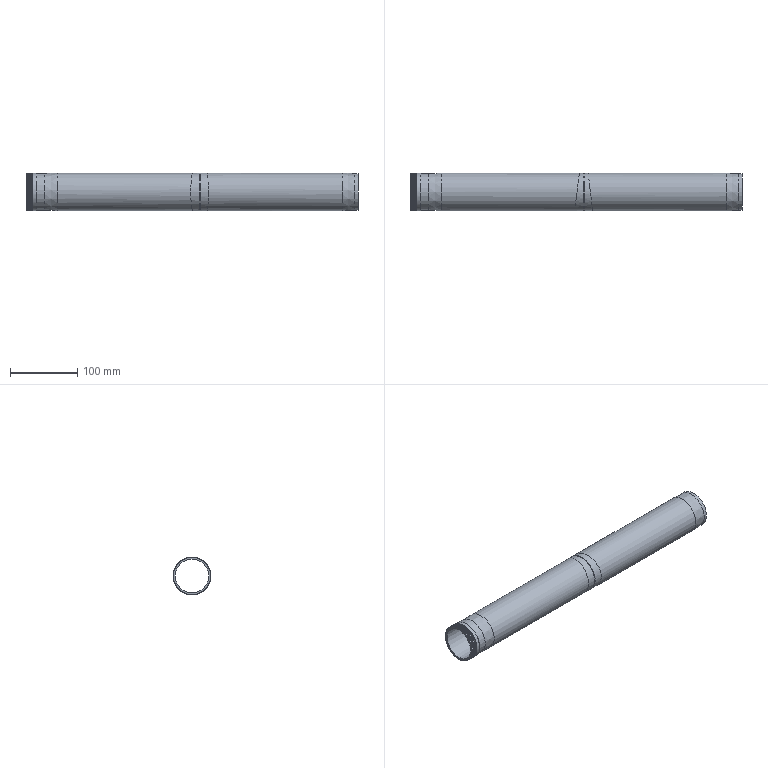Part | STEP file | PN_0083_default | 1 solid | 1364 faces | box 495 x 56 x 56 mm | volume 244128 mm3 | plane 1353 | cylinder 9 | cone 2 | commonest cylinder face diameters 56 x6 55.031 x2 50 x1